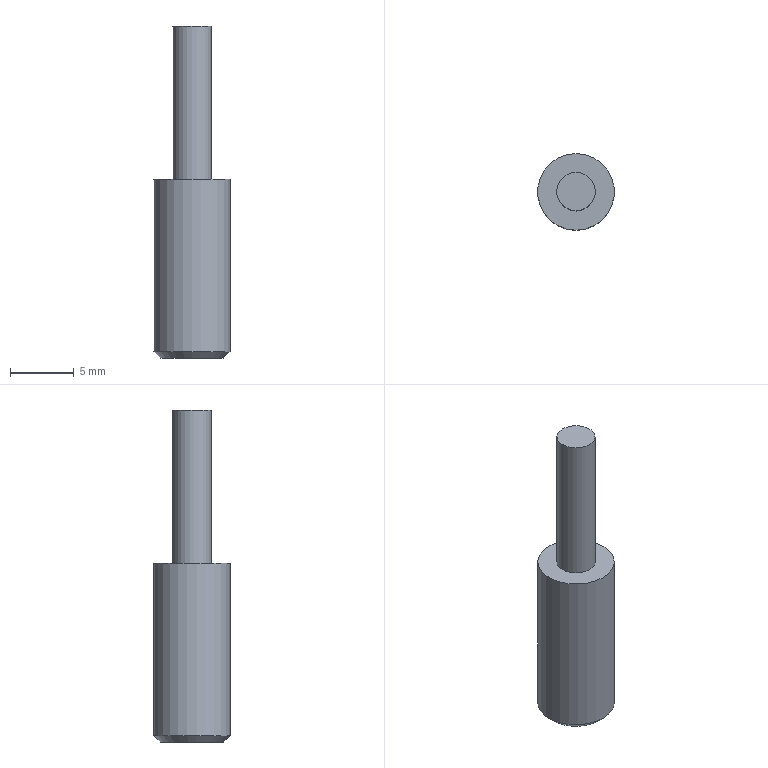Part | STEP file | 1-41.6 | 1 solid | 6 faces | box 6 x 6 x 26 mm | volume 478.438 mm3 | plane 3 | cylinder 2 | cone 1 | commonest cylinder face diameters 3 x1 6 x1
STEP:
#1=CARTESIAN_POINT('',(0.,0.,0.));
#2=DIRECTION('',(0.,0.,1.));
#3=DIRECTION('',(1.,0.,0.));
#4=AXIS2_PLACEMENT_3D('',#1,#2,#3);
#5=CARTESIAN_POINT('',(0.,1.5,12.));
#6=VERTEX_POINT('',#5);
#7=CARTESIAN_POINT('',(0.,0.,12.));
#8=DIRECTION('',(0.,0.,1.));
#9=DIRECTION('',(0.,1.,0.));
#10=AXIS2_PLACEMENT_3D('',#7,#8,#9);
#11=CIRCLE('',#10,1.5);
#12=CARTESIAN_POINT('',(0.,-0.4019,12.));
#13=DIRECTION('',(0.,0.,1.));
#14=DIRECTION('',(1.,0.,0.));
#15=AXIS2_PLACEMENT_3D('',#12,#13,#14);
#16=PLANE('',#15);
#17=CARTESIAN_POINT('',(0.,0.4019));
#18=DIRECTION('',(0.,1.));
#19=AXIS2_PLACEMENT_2D('',#17,#18);
#20=CIRCLE('',#19,1.5);
#21=(GEOMETRIC_REPRESENTATION_CONTEXT(2)PARAMETRIC_REPRESENTATION_CONTEXT()REPRESENTATION_CONTEXT('',''));
#22=DEFINITIONAL_REPRESENTATION('',(#20),#21);
#23=PCURVE('',#16,#22);
#24=CARTESIAN_POINT('',(0.,0.,0.));
#25=DIRECTION('',(0.,0.,1.));
#26=DIRECTION('',(0.,1.,0.));
#27=AXIS2_PLACEMENT_3D('',#24,#25,#26);
#28=CYLINDRICAL_SURFACE('',#27,1.5);
#29=CARTESIAN_POINT('',(0.,12.));
#30=DIRECTION('',(1.,0.));
#31=VECTOR('',#30,1.);
#32=LINE('',#29,#31);
#33=(GEOMETRIC_REPRESENTATION_CONTEXT(2)PARAMETRIC_REPRESENTATION_CONTEXT()REPRESENTATION_CONTEXT('',''));
#34=DEFINITIONAL_REPRESENTATION('',(#32),#33);
#35=PCURVE('',#28,#34);
#36=SURFACE_CURVE('',#11,(#23,#35),.PCURVE_S1.);
#37=EDGE_CURVE('',#6,#6,#36,.T.);
#38=ORIENTED_EDGE('',*,*,#37,.T.);
#39=EDGE_LOOP('',(#38));
#40=FACE_BOUND('',#39,.T.);
#41=ADVANCED_FACE('',(#40),#16,.T.);
#42=CARTESIAN_POINT('',(0.,1.5,0.));
#43=VERTEX_POINT('',#42);
#44=CARTESIAN_POINT('',(0.,0.,0.));
#45=DIRECTION('',(0.,0.,1.));
#46=DIRECTION('',(0.,1.,0.));
#47=AXIS2_PLACEMENT_3D('',#44,#45,#46);
#48=CIRCLE('',#47,1.5);
#49=CARTESIAN_POINT('',(0.,0.));
#50=DIRECTION('',(1.,0.));
#51=VECTOR('',#50,1.);
#52=LINE('',#49,#51);
#53=(GEOMETRIC_REPRESENTATION_CONTEXT(2)PARAMETRIC_REPRESENTATION_CONTEXT()REPRESENTATION_CONTEXT('',''));
#54=DEFINITIONAL_REPRESENTATION('',(#52),#53);
#55=PCURVE('',#28,#54);
#56=CARTESIAN_POINT('',(0.,-0.8038,0.));
#57=DIRECTION('',(0.,0.,1.));
#58=DIRECTION('',(1.,0.,0.));
#59=AXIS2_PLACEMENT_3D('',#56,#57,#58);
#60=PLANE('',#59);
#61=CARTESIAN_POINT('',(0.,0.8038));
#62=DIRECTION('',(0.,1.));
#63=AXIS2_PLACEMENT_2D('',#61,#62);
#64=CIRCLE('',#63,1.5);
#65=(GEOMETRIC_REPRESENTATION_CONTEXT(2)PARAMETRIC_REPRESENTATION_CONTEXT()REPRESENTATION_CONTEXT('',''));
#66=DEFINITIONAL_REPRESENTATION('',(#64),#65);
#67=PCURVE('',#60,#66);
#68=SURFACE_CURVE('',#48,(#55,#67),.PCURVE_S1.);
#69=EDGE_CURVE('',#43,#43,#68,.T.);
#70=ORIENTED_EDGE('',*,*,#69,.T.);
#71=CARTESIAN_POINT('',(0.,1.5,0.));
#72=DIRECTION('',(0.,0.,1.));
#73=VECTOR('',#72,1.);
#74=LINE('',#71,#73);
#75=CARTESIAN_POINT('',(6.283,0.));
#76=DIRECTION('',(0.,1.));
#77=VECTOR('',#76,1.);
#78=LINE('',#75,#77);
#79=(GEOMETRIC_REPRESENTATION_CONTEXT(2)PARAMETRIC_REPRESENTATION_CONTEXT()REPRESENTATION_CONTEXT('',''));
#80=DEFINITIONAL_REPRESENTATION('',(#78),#79);
#81=PCURVE('',#28,#80);
#82=CARTESIAN_POINT('',(0.,0.));
#83=DIRECTION('',(0.,1.));
#84=VECTOR('',#83,1.);
#85=LINE('',#82,#84);
#86=(GEOMETRIC_REPRESENTATION_CONTEXT(2)PARAMETRIC_REPRESENTATION_CONTEXT()REPRESENTATION_CONTEXT('',''));
#87=DEFINITIONAL_REPRESENTATION('',(#85),#86);
#88=PCURVE('',#28,#87);
#89=SEAM_CURVE('',#74,(#81,#88),.PCURVE_S1.);
#90=EDGE_CURVE('',#43,#6,#89,.T.);
#91=ORIENTED_EDGE('',*,*,#90,.T.);
#92=ORIENTED_EDGE('',*,*,#37,.F.);
#93=ORIENTED_EDGE('',*,*,#90,.F.);
#94=EDGE_LOOP('',(#70,#91,#92,#93));
#95=FACE_BOUND('',#94,.T.);
#96=ADVANCED_FACE('',(#95),#28,.T.);
#97=CARTESIAN_POINT('',(0.,3.,0.));
#98=VERTEX_POINT('',#97);
#99=CARTESIAN_POINT('',(0.,0.,0.));
#100=DIRECTION('',(0.,0.,1.));
#101=DIRECTION('',(0.,1.,0.));
#102=AXIS2_PLACEMENT_3D('',#99,#100,#101);
#103=CIRCLE('',#102,3.);
#104=CARTESIAN_POINT('',(0.,0.8038));
#105=DIRECTION('',(0.,1.));
#106=AXIS2_PLACEMENT_2D('',#104,#105);
#107=CIRCLE('',#106,3.);
#108=(GEOMETRIC_REPRESENTATION_CONTEXT(2)PARAMETRIC_REPRESENTATION_CONTEXT()REPRESENTATION_CONTEXT('',''));
#109=DEFINITIONAL_REPRESENTATION('',(#107),#108);
#110=PCURVE('',#60,#109);
#111=CARTESIAN_POINT('',(0.,0.,0.));
#112=DIRECTION('',(0.,0.,-1.));
#113=DIRECTION('',(0.,1.,0.));
#114=AXIS2_PLACEMENT_3D('',#111,#112,#113);
#115=CYLINDRICAL_SURFACE('',#114,3.);
#116=CARTESIAN_POINT('',(6.283,0.));
#117=DIRECTION('',(-1.,0.));
#118=VECTOR('',#117,1.);
#119=LINE('',#116,#118);
#120=(GEOMETRIC_REPRESENTATION_CONTEXT(2)PARAMETRIC_REPRESENTATION_CONTEXT()REPRESENTATION_CONTEXT('',''));
#121=DEFINITIONAL_REPRESENTATION('',(#119),#120);
#122=PCURVE('',#115,#121);
#123=SURFACE_CURVE('',#103,(#110,#122),.PCURVE_S1.);
#124=EDGE_CURVE('',#98,#98,#123,.T.);
#125=ORIENTED_EDGE('',*,*,#124,.T.);
#126=EDGE_LOOP('',(#125));
#127=FACE_BOUND('',#126,.T.);
#128=ORIENTED_EDGE('',*,*,#69,.F.);
#129=EDGE_LOOP('',(#128));
#130=FACE_BOUND('',#129,.T.);
#131=ADVANCED_FACE('',(#127,#130),#60,.T.);
#132=CARTESIAN_POINT('',(0.,3.,-13.5));
#133=VERTEX_POINT('',#132);
#134=CARTESIAN_POINT('',(0.,3.,0.));
#135=DIRECTION('',(0.,0.,-1.));
#136=VECTOR('',#135,1.);
#137=LINE('',#134,#136);
#138=CARTESIAN_POINT('',(6.283,0.));
#139=DIRECTION('',(0.,1.));
#140=VECTOR('',#139,1.);
#141=LINE('',#138,#140);
#142=(GEOMETRIC_REPRESENTATION_CONTEXT(2)PARAMETRIC_REPRESENTATION_CONTEXT()REPRESENTATION_CONTEXT('',''));
#143=DEFINITIONAL_REPRESENTATION('',(#141),#142);
#144=PCURVE('',#115,#143);
#145=CARTESIAN_POINT('',(0.,0.));
#146=DIRECTION('',(0.,1.));
#147=VECTOR('',#146,1.);
#148=LINE('',#145,#147);
#149=(GEOMETRIC_REPRESENTATION_CONTEXT(2)PARAMETRIC_REPRESENTATION_CONTEXT()REPRESENTATION_CONTEXT('',''));
#150=DEFINITIONAL_REPRESENTATION('',(#148),#149);
#151=PCURVE('',#115,#150);
#152=SEAM_CURVE('',#137,(#144,#151),.PCURVE_S1.);
#153=EDGE_CURVE('',#98,#133,#152,.T.);
#154=ORIENTED_EDGE('',*,*,#153,.T.);
#155=CARTESIAN_POINT('',(0.,0.,-13.5));
#156=DIRECTION('',(0.,0.,1.));
#157=DIRECTION('',(0.,1.,0.));
#158=AXIS2_PLACEMENT_3D('',#155,#156,#157);
#159=CIRCLE('',#158,3.);
#160=CARTESIAN_POINT('',(6.283,13.5));
#161=DIRECTION('',(-1.,0.));
#162=VECTOR('',#161,1.);
#163=LINE('',#160,#162);
#164=(GEOMETRIC_REPRESENTATION_CONTEXT(2)PARAMETRIC_REPRESENTATION_CONTEXT()REPRESENTATION_CONTEXT('',''));
#165=DEFINITIONAL_REPRESENTATION('',(#163),#164);
#166=PCURVE('',#115,#165);
#167=CARTESIAN_POINT('',(0.,0.,-14.));
#168=DIRECTION('',(0.,0.,1.));
#169=DIRECTION('',(0.,1.,0.));
#170=AXIS2_PLACEMENT_3D('',#167,#168,#169);
#171=CONICAL_SURFACE('',#170,2.5,0.7854);
#172=CARTESIAN_POINT('',(0.,0.5));
#173=DIRECTION('',(1.,0.));
#174=VECTOR('',#173,1.);
#175=LINE('',#172,#174);
#176=(GEOMETRIC_REPRESENTATION_CONTEXT(2)PARAMETRIC_REPRESENTATION_CONTEXT()REPRESENTATION_CONTEXT('',''));
#177=DEFINITIONAL_REPRESENTATION('',(#175),#176);
#178=PCURVE('',#171,#177);
#179=SURFACE_CURVE('',#159,(#166,#178),.PCURVE_S1.);
#180=EDGE_CURVE('',#133,#133,#179,.T.);
#181=ORIENTED_EDGE('',*,*,#180,.T.);
#182=ORIENTED_EDGE('',*,*,#153,.F.);
#183=ORIENTED_EDGE('',*,*,#124,.F.);
#184=EDGE_LOOP('',(#154,#181,#182,#183));
#185=FACE_BOUND('',#184,.T.);
#186=ADVANCED_FACE('',(#185),#115,.T.);
#187=CARTESIAN_POINT('',(0.,2.5,-14.));
#188=VERTEX_POINT('',#187);
#189=CARTESIAN_POINT('',(0.,0.,-14.));
#190=DIRECTION('',(0.,0.,1.));
#191=DIRECTION('',(0.,1.,0.));
#192=AXIS2_PLACEMENT_3D('',#189,#190,#191);
#193=CIRCLE('',#192,2.5);
#194=CARTESIAN_POINT('',(0.,-0.8038,-14.));
#195=DIRECTION('',(0.,0.,1.));
#196=DIRECTION('',(1.,0.,0.));
#197=AXIS2_PLACEMENT_3D('',#194,#195,#196);
#198=PLANE('',#197);
#199=CARTESIAN_POINT('',(0.,0.8038));
#200=DIRECTION('',(0.,1.));
#201=AXIS2_PLACEMENT_2D('',#199,#200);
#202=CIRCLE('',#201,2.5);
#203=(GEOMETRIC_REPRESENTATION_CONTEXT(2)PARAMETRIC_REPRESENTATION_CONTEXT()REPRESENTATION_CONTEXT('',''));
#204=DEFINITIONAL_REPRESENTATION('',(#202),#203);
#205=PCURVE('',#198,#204);
#206=CARTESIAN_POINT('',(0.,0.));
#207=DIRECTION('',(1.,0.));
#208=VECTOR('',#207,1.);
#209=LINE('',#206,#208);
#210=(GEOMETRIC_REPRESENTATION_CONTEXT(2)PARAMETRIC_REPRESENTATION_CONTEXT()REPRESENTATION_CONTEXT('',''));
#211=DEFINITIONAL_REPRESENTATION('',(#209),#210);
#212=PCURVE('',#171,#211);
#213=SURFACE_CURVE('',#193,(#205,#212),.PCURVE_S1.);
#214=EDGE_CURVE('',#188,#188,#213,.T.);
#215=ORIENTED_EDGE('',*,*,#214,.T.);
#216=EDGE_LOOP('',(#215));
#217=FACE_BOUND('',#216,.F.);
#218=ADVANCED_FACE('',(#217),#198,.F.);
#219=CARTESIAN_POINT('',(0.,2.5,-14.));
#220=DIRECTION('',(0.,0.7071,0.7071));
#221=VECTOR('',#220,1.);
#222=LINE('',#219,#221);
#223=CARTESIAN_POINT('',(6.283,0.));
#224=DIRECTION('',(0.,1.));
#225=VECTOR('',#224,1.);
#226=LINE('',#223,#225);
#227=(GEOMETRIC_REPRESENTATION_CONTEXT(2)PARAMETRIC_REPRESENTATION_CONTEXT()REPRESENTATION_CONTEXT('',''));
#228=DEFINITIONAL_REPRESENTATION('',(#226),#227);
#229=PCURVE('',#171,#228);
#230=CARTESIAN_POINT('',(0.,0.));
#231=DIRECTION('',(0.,1.));
#232=VECTOR('',#231,1.);
#233=LINE('',#230,#232);
#234=(GEOMETRIC_REPRESENTATION_CONTEXT(2)PARAMETRIC_REPRESENTATION_CONTEXT()REPRESENTATION_CONTEXT('',''));
#235=DEFINITIONAL_REPRESENTATION('',(#233),#234);
#236=PCURVE('',#171,#235);
#237=SEAM_CURVE('',#222,(#229,#236),.PCURVE_S1.);
#238=EDGE_CURVE('',#188,#133,#237,.T.);
#239=ORIENTED_EDGE('',*,*,#238,.T.);
#240=ORIENTED_EDGE('',*,*,#180,.F.);
#241=ORIENTED_EDGE('',*,*,#238,.F.);
#242=ORIENTED_EDGE('',*,*,#214,.T.);
#243=EDGE_LOOP('',(#239,#240,#241,#242));
#244=FACE_BOUND('',#243,.T.);
#245=ADVANCED_FACE('',(#244),#171,.T.);
#246=CLOSED_SHELL('',(#41,#96,#131,#186,#218,#245));
#247=MANIFOLD_SOLID_BREP('',#246);
#248=(LENGTH_UNIT()NAMED_UNIT(*)SI_UNIT(.MILLI.,.METRE.));
#249=UNCERTAINTY_MEASURE_WITH_UNIT(LENGTH_MEASURE(0.0000001),#248,'','');
#250=(NAMED_UNIT(*)PLANE_ANGLE_UNIT()SI_UNIT($,.RADIAN.));
#251=(NAMED_UNIT(*)SI_UNIT($,.STERADIAN.)SOLID_ANGLE_UNIT());
#252=(GEOMETRIC_REPRESENTATION_CONTEXT(3)GLOBAL_UNCERTAINTY_ASSIGNED_CONTEXT((#249))GLOBAL_UNIT_ASSIGNED_CONTEXT((#248,#250,#251))REPRESENTATION_CONTEXT('',''));
#253=ADVANCED_BREP_SHAPE_REPRESENTATION('',(#4,#247),#252);